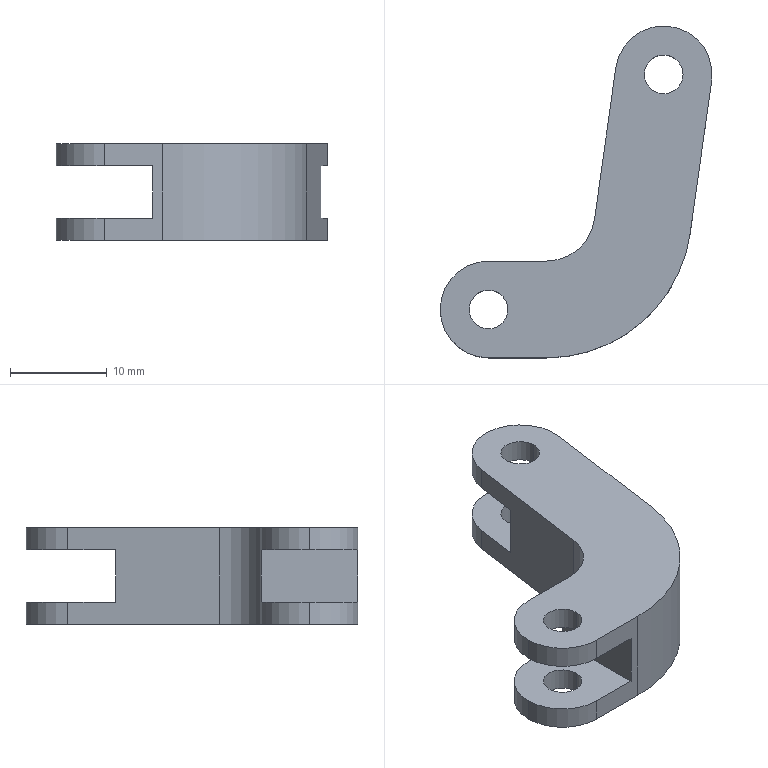Part | SolidWorks | features ICE 4, Extrusion 1 | 1 solid | 28 faces | box 28.109 x 34.304 x 10 mm | volume 3322 mm3 | cylinder 16 | plane 12 | commonest cylinder face diameters 4 x8 10 x7 30 x1
STEP:
#1=CARTESIAN_POINT('',(20.109,19.304,2.7));
#2=VERTEX_POINT('',#1);
#3=CARTESIAN_POINT('',(16.109,19.304,2.7));
#4=VERTEX_POINT('',#3);
#5=CARTESIAN_POINT('',(18.109,19.304,2.7));
#6=DIRECTION('',(0.,0.,-1.));
#7=DIRECTION('',(0.,-1.,0.));
#8=AXIS2_PLACEMENT_3D('',#5,#6,#7);
#9=CIRCLE('',#8,2.);
#10=EDGE_CURVE('',#2,#4,#9,.T.);
#11=ORIENTED_EDGE('',*,*,#10,.T.);
#12=CARTESIAN_POINT('',(16.109,19.304,5.));
#13=VERTEX_POINT('',#12);
#14=CARTESIAN_POINT('',(16.109,19.304,-26.));
#15=DIRECTION('',(0.,0.,1.));
#16=VECTOR('',#15,1000.);
#17=LINE('',#14,#16);
#18=EDGE_CURVE('',#4,#13,#17,.T.);
#19=ORIENTED_EDGE('',*,*,#18,.T.);
#20=CARTESIAN_POINT('',(20.109,19.304,5.));
#21=VERTEX_POINT('',#20);
#22=CARTESIAN_POINT('',(18.109,19.304,5.));
#23=DIRECTION('',(0.,0.,1.));
#24=DIRECTION('',(1.,0.,0.));
#25=AXIS2_PLACEMENT_3D('',#22,#23,#24);
#26=CIRCLE('',#25,2.);
#27=EDGE_CURVE('',#13,#21,#26,.T.);
#28=ORIENTED_EDGE('',*,*,#27,.T.);
#29=CARTESIAN_POINT('',(20.109,19.304,-26.));
#30=DIRECTION('',(0.,0.,1.));
#31=VECTOR('',#30,1000.);
#32=LINE('',#29,#31);
#33=EDGE_CURVE('',#2,#21,#32,.T.);
#34=ORIENTED_EDGE('',*,*,#33,.F.);
#35=EDGE_LOOP('',(#11,#19,#28,#34));
#36=FACE_OUTER_BOUND('',#35,.T.);
#37=CARTESIAN_POINT('',(18.109,19.304,-26.));
#38=DIRECTION('',(0.,0.,1.));
#39=DIRECTION('',(1.,0.,0.));
#40=AXIS2_PLACEMENT_3D('',#37,#38,#39);
#41=CYLINDRICAL_SURFACE('',#40,2.);
#42=ADVANCED_FACE('',(#36),#41,.F.);
#43=CARTESIAN_POINT('',(-2.,-5.,2.7));
#44=VERTEX_POINT('',#43);
#45=CARTESIAN_POINT('',(2.,-5.,2.7));
#46=VERTEX_POINT('',#45);
#47=CARTESIAN_POINT('',(0.,-5.,2.7));
#48=DIRECTION('',(0.,0.,1.));
#49=DIRECTION('',(0.,1.,0.));
#50=AXIS2_PLACEMENT_3D('',#47,#48,#49);
#51=CIRCLE('',#50,2.);
#52=EDGE_CURVE('',#44,#46,#51,.T.);
#53=ORIENTED_EDGE('',*,*,#52,.F.);
#54=CARTESIAN_POINT('',(-2.,-5.,5.));
#55=VERTEX_POINT('',#54);
#56=CARTESIAN_POINT('',(-2.,-5.,-5.));
#57=DIRECTION('',(0.,0.,1.));
#58=VECTOR('',#57,1000.);
#59=LINE('',#56,#58);
#60=EDGE_CURVE('',#44,#55,#59,.T.);
#61=ORIENTED_EDGE('',*,*,#60,.T.);
#62=CARTESIAN_POINT('',(2.,-5.,5.));
#63=VERTEX_POINT('',#62);
#64=CARTESIAN_POINT('',(0.,-5.,5.));
#65=DIRECTION('',(0.,0.,1.));
#66=DIRECTION('',(1.,0.,0.));
#67=AXIS2_PLACEMENT_3D('',#64,#65,#66);
#68=CIRCLE('',#67,2.);
#69=EDGE_CURVE('',#55,#63,#68,.T.);
#70=ORIENTED_EDGE('',*,*,#69,.T.);
#71=CARTESIAN_POINT('',(2.,-5.,-5.));
#72=DIRECTION('',(0.,0.,1.));
#73=VECTOR('',#72,1000.);
#74=LINE('',#71,#73);
#75=EDGE_CURVE('',#46,#63,#74,.T.);
#76=ORIENTED_EDGE('',*,*,#75,.F.);
#77=EDGE_LOOP('',(#53,#61,#70,#76));
#78=FACE_OUTER_BOUND('',#77,.T.);
#79=CARTESIAN_POINT('',(0.,-5.,-5.));
#80=DIRECTION('',(0.,0.,1.));
#81=DIRECTION('',(1.,0.,0.));
#82=AXIS2_PLACEMENT_3D('',#79,#80,#81);
#83=CYLINDRICAL_SURFACE('',#82,2.);
#84=ADVANCED_FACE('',(#78),#83,.F.);
#85=CARTESIAN_POINT('',(-2.,-5.,-5.));
#86=VERTEX_POINT('',#85);
#87=CARTESIAN_POINT('',(2.,-5.,-5.));
#88=VERTEX_POINT('',#87);
#89=CARTESIAN_POINT('',(0.,-5.,-5.));
#90=DIRECTION('',(0.,0.,1.));
#91=DIRECTION('',(1.,0.,0.));
#92=AXIS2_PLACEMENT_3D('',#89,#90,#91);
#93=CIRCLE('',#92,2.);
#94=EDGE_CURVE('',#86,#88,#93,.T.);
#95=ORIENTED_EDGE('',*,*,#94,.F.);
#96=CARTESIAN_POINT('',(-2.,-5.,-2.7));
#97=VERTEX_POINT('',#96);
#98=CARTESIAN_POINT('',(-2.,-5.,-5.));
#99=DIRECTION('',(0.,0.,1.));
#100=VECTOR('',#99,1000.);
#101=LINE('',#98,#100);
#102=EDGE_CURVE('',#86,#97,#101,.T.);
#103=ORIENTED_EDGE('',*,*,#102,.T.);
#104=CARTESIAN_POINT('',(2.,-5.,-2.7));
#105=VERTEX_POINT('',#104);
#106=CARTESIAN_POINT('',(0.,-5.,-2.7));
#107=DIRECTION('',(0.,0.,-1.));
#108=DIRECTION('',(0.,-1.,0.));
#109=AXIS2_PLACEMENT_3D('',#106,#107,#108);
#110=CIRCLE('',#109,2.);
#111=EDGE_CURVE('',#105,#97,#110,.T.);
#112=ORIENTED_EDGE('',*,*,#111,.F.);
#113=CARTESIAN_POINT('',(2.,-5.,-5.));
#114=DIRECTION('',(0.,0.,1.));
#115=VECTOR('',#114,1000.);
#116=LINE('',#113,#115);
#117=EDGE_CURVE('',#88,#105,#116,.T.);
#118=ORIENTED_EDGE('',*,*,#117,.F.);
#119=EDGE_LOOP('',(#95,#103,#112,#118));
#120=FACE_OUTER_BOUND('',#119,.T.);
#121=CARTESIAN_POINT('',(0.,-5.,-5.));
#122=DIRECTION('',(0.,0.,1.));
#123=DIRECTION('',(1.,0.,0.));
#124=AXIS2_PLACEMENT_3D('',#121,#122,#123);
#125=CYLINDRICAL_SURFACE('',#124,2.);
#126=ADVANCED_FACE('',(#120),#125,.F.);
#127=CARTESIAN_POINT('',(-5.,-5.,5.));
#128=VERTEX_POINT('',#127);
#129=CARTESIAN_POINT('',(0.,-10.,5.));
#130=VERTEX_POINT('',#129);
#131=CARTESIAN_POINT('',(0.,-5.,5.));
#132=DIRECTION('',(0.,0.,1.));
#133=DIRECTION('',(1.,0.,0.));
#134=AXIS2_PLACEMENT_3D('',#131,#132,#133);
#135=CIRCLE('',#134,5.);
#136=EDGE_CURVE('',#128,#130,#135,.T.);
#137=ORIENTED_EDGE('',*,*,#136,.F.);
#138=CARTESIAN_POINT('',(-5.,-5.,2.7));
#139=VERTEX_POINT('',#138);
#140=CARTESIAN_POINT('',(-5.,-5.,5.));
#141=DIRECTION('',(0.,0.,-1.));
#142=VECTOR('',#141,1000.);
#143=LINE('',#140,#142);
#144=EDGE_CURVE('',#128,#139,#143,.T.);
#145=ORIENTED_EDGE('',*,*,#144,.T.);
#146=CARTESIAN_POINT('',(0.,-10.,2.7));
#147=VERTEX_POINT('',#146);
#148=CARTESIAN_POINT('',(0.,-5.,2.7));
#149=DIRECTION('',(0.,0.,-1.));
#150=DIRECTION('',(0.,1.,0.));
#151=AXIS2_PLACEMENT_3D('',#148,#149,#150);
#152=CIRCLE('',#151,5.);
#153=EDGE_CURVE('',#147,#139,#152,.T.);
#154=ORIENTED_EDGE('',*,*,#153,.F.);
#155=CARTESIAN_POINT('',(0.,-10.,5.));
#156=DIRECTION('',(0.,0.,-1.));
#157=VECTOR('',#156,1000.);
#158=LINE('',#155,#157);
#159=EDGE_CURVE('',#130,#147,#158,.T.);
#160=ORIENTED_EDGE('',*,*,#159,.F.);
#161=EDGE_LOOP('',(#137,#145,#154,#160));
#162=FACE_OUTER_BOUND('',#161,.T.);
#163=CARTESIAN_POINT('',(0.,-5.,5.));
#164=DIRECTION('',(0.,0.,-1.));
#165=DIRECTION('',(-1.,0.,0.));
#166=AXIS2_PLACEMENT_3D('',#163,#164,#165);
#167=CYLINDRICAL_SURFACE('',#166,5.);
#168=ADVANCED_FACE('',(#162),#167,.T.);
#169=CARTESIAN_POINT('',(-5.,-5.,-2.7));
#170=VERTEX_POINT('',#169);
#171=CARTESIAN_POINT('',(0.,-10.,-2.7));
#172=VERTEX_POINT('',#171);
#173=CARTESIAN_POINT('',(0.,-5.,-2.7));
#174=DIRECTION('',(0.,0.,1.));
#175=DIRECTION('',(0.,-1.,0.));
#176=AXIS2_PLACEMENT_3D('',#173,#174,#175);
#177=CIRCLE('',#176,5.);
#178=EDGE_CURVE('',#170,#172,#177,.T.);
#179=ORIENTED_EDGE('',*,*,#178,.F.);
#180=CARTESIAN_POINT('',(-5.,-5.,-5.));
#181=VERTEX_POINT('',#180);
#182=CARTESIAN_POINT('',(-5.,-5.,5.));
#183=DIRECTION('',(0.,0.,-1.));
#184=VECTOR('',#183,1000.);
#185=LINE('',#182,#184);
#186=EDGE_CURVE('',#170,#181,#185,.T.);
#187=ORIENTED_EDGE('',*,*,#186,.T.);
#188=CARTESIAN_POINT('',(0.,-10.,-5.));
#189=VERTEX_POINT('',#188);
#190=CARTESIAN_POINT('',(0.,-5.,-5.));
#191=DIRECTION('',(0.,0.,1.));
#192=DIRECTION('',(1.,0.,0.));
#193=AXIS2_PLACEMENT_3D('',#190,#191,#192);
#194=CIRCLE('',#193,5.);
#195=EDGE_CURVE('',#181,#189,#194,.T.);
#196=ORIENTED_EDGE('',*,*,#195,.T.);
#197=CARTESIAN_POINT('',(0.,-10.,5.));
#198=DIRECTION('',(0.,0.,-1.));
#199=VECTOR('',#198,1000.);
#200=LINE('',#197,#199);
#201=EDGE_CURVE('',#172,#189,#200,.T.);
#202=ORIENTED_EDGE('',*,*,#201,.F.);
#203=EDGE_LOOP('',(#179,#187,#196,#202));
#204=FACE_OUTER_BOUND('',#203,.T.);
#205=CARTESIAN_POINT('',(0.,-5.,5.));
#206=DIRECTION('',(0.,0.,-1.));
#207=DIRECTION('',(-1.,0.,0.));
#208=AXIS2_PLACEMENT_3D('',#205,#206,#207);
#209=CYLINDRICAL_SURFACE('',#208,5.);
#210=ADVANCED_FACE('',(#204),#209,.T.);
#211=CARTESIAN_POINT('',(16.109,19.304,-5.));
#212=VERTEX_POINT('',#211);
#213=CARTESIAN_POINT('',(20.109,19.304,-5.));
#214=VERTEX_POINT('',#213);
#215=CARTESIAN_POINT('',(18.109,19.304,-5.));
#216=DIRECTION('',(0.,0.,1.));
#217=DIRECTION('',(1.,0.,0.));
#218=AXIS2_PLACEMENT_3D('',#215,#216,#217);
#219=CIRCLE('',#218,2.);
#220=EDGE_CURVE('',#212,#214,#219,.T.);
#221=ORIENTED_EDGE('',*,*,#220,.F.);
#222=CARTESIAN_POINT('',(16.109,19.304,-2.7));
#223=VERTEX_POINT('',#222);
#224=CARTESIAN_POINT('',(16.109,19.304,-26.));
#225=DIRECTION('',(0.,0.,1.));
#226=VECTOR('',#225,1000.);
#227=LINE('',#224,#226);
#228=EDGE_CURVE('',#212,#223,#227,.T.);
#229=ORIENTED_EDGE('',*,*,#228,.T.);
#230=CARTESIAN_POINT('',(20.109,19.304,-2.7));
#231=VERTEX_POINT('',#230);
#232=CARTESIAN_POINT('',(18.109,19.304,-2.7));
#233=DIRECTION('',(0.,0.,1.));
#234=DIRECTION('',(0.,1.,0.));
#235=AXIS2_PLACEMENT_3D('',#232,#233,#234);
#236=CIRCLE('',#235,2.);
#237=EDGE_CURVE('',#223,#231,#236,.T.);
#238=ORIENTED_EDGE('',*,*,#237,.T.);
#239=CARTESIAN_POINT('',(20.109,19.304,-26.));
#240=DIRECTION('',(0.,0.,1.));
#241=VECTOR('',#240,1000.);
#242=LINE('',#239,#241);
#243=EDGE_CURVE('',#214,#231,#242,.T.);
#244=ORIENTED_EDGE('',*,*,#243,.F.);
#245=EDGE_LOOP('',(#221,#229,#238,#244));
#246=FACE_OUTER_BOUND('',#245,.T.);
#247=CARTESIAN_POINT('',(18.109,19.304,-26.));
#248=DIRECTION('',(0.,0.,1.));
#249=DIRECTION('',(1.,0.,0.));
#250=AXIS2_PLACEMENT_3D('',#247,#248,#249);
#251=CYLINDRICAL_SURFACE('',#250,2.);
#252=ADVANCED_FACE('',(#246),#251,.F.);
#253=CARTESIAN_POINT('',(13.157,20.,-2.7));
#254=VERTEX_POINT('',#253);
#255=CARTESIAN_POINT('',(23.06,18.608,-2.7));
#256=VERTEX_POINT('',#255);
#257=CARTESIAN_POINT('',(18.109,19.304,-2.7));
#258=DIRECTION('',(0.,0.,-1.));
#259=DIRECTION('',(0.,1.,0.));
#260=AXIS2_PLACEMENT_3D('',#257,#258,#259);
#261=CIRCLE('',#260,5.);
#262=EDGE_CURVE('',#254,#256,#261,.T.);
#263=ORIENTED_EDGE('',*,*,#262,.T.);
#264=CARTESIAN_POINT('',(23.06,18.608,-5.));
#265=VERTEX_POINT('',#264);
#266=CARTESIAN_POINT('',(23.06,18.608,5.));
#267=DIRECTION('',(0.,0.,-1.));
#268=VECTOR('',#267,1000.);
#269=LINE('',#266,#268);
#270=EDGE_CURVE('',#256,#265,#269,.T.);
#271=ORIENTED_EDGE('',*,*,#270,.T.);
#272=CARTESIAN_POINT('',(13.157,20.,-5.));
#273=VERTEX_POINT('',#272);
#274=CARTESIAN_POINT('',(18.109,19.304,-5.));
#275=DIRECTION('',(0.,0.,1.));
#276=DIRECTION('',(-1.,0.,0.));
#277=AXIS2_PLACEMENT_3D('',#274,#275,#276);
#278=CIRCLE('',#277,5.);
#279=EDGE_CURVE('',#265,#273,#278,.T.);
#280=ORIENTED_EDGE('',*,*,#279,.T.);
#281=CARTESIAN_POINT('',(13.157,20.,5.));
#282=DIRECTION('',(0.,0.,-1.));
#283=VECTOR('',#282,1000.);
#284=LINE('',#281,#283);
#285=EDGE_CURVE('',#254,#273,#284,.T.);
#286=ORIENTED_EDGE('',*,*,#285,.F.);
#287=EDGE_LOOP('',(#263,#271,#280,#286));
#288=FACE_OUTER_BOUND('',#287,.T.);
#289=CARTESIAN_POINT('',(18.109,19.304,5.));
#290=DIRECTION('',(0.,0.,-1.));
#291=DIRECTION('',(-1.,0.,0.));
#292=AXIS2_PLACEMENT_3D('',#289,#290,#291);
#293=CYLINDRICAL_SURFACE('',#292,5.);
#294=ADVANCED_FACE('',(#288),#293,.T.);
#295=ORIENTED_EDGE('',*,*,#228,.F.);
#296=CARTESIAN_POINT('',(18.109,19.304,-5.));
#297=DIRECTION('',(0.,0.,1.));
#298=DIRECTION('',(1.,0.,0.));
#299=AXIS2_PLACEMENT_3D('',#296,#297,#298);
#300=CIRCLE('',#299,2.);
#301=EDGE_CURVE('',#214,#212,#300,.T.);
#302=ORIENTED_EDGE('',*,*,#301,.F.);
#303=ORIENTED_EDGE('',*,*,#243,.T.);
#304=CARTESIAN_POINT('',(18.109,19.304,-2.7));
#305=DIRECTION('',(0.,0.,1.));
#306=DIRECTION('',(0.,1.,0.));
#307=AXIS2_PLACEMENT_3D('',#304,#305,#306);
#308=CIRCLE('',#307,2.);
#309=EDGE_CURVE('',#231,#223,#308,.T.);
#310=ORIENTED_EDGE('',*,*,#309,.T.);
#311=EDGE_LOOP('',(#295,#302,#303,#310));
#312=FACE_OUTER_BOUND('',#311,.T.);
#313=CARTESIAN_POINT('',(18.109,19.304,-26.));
#314=DIRECTION('',(0.,0.,1.));
#315=DIRECTION('',(1.,0.,0.));
#316=AXIS2_PLACEMENT_3D('',#313,#314,#315);
#317=CYLINDRICAL_SURFACE('',#316,2.);
#318=ADVANCED_FACE('',(#312),#317,.F.);
#319=CARTESIAN_POINT('',(5.,0.,-2.7));
#320=VERTEX_POINT('',#319);
#321=CARTESIAN_POINT('',(0.,0.,-2.7));
#322=VERTEX_POINT('',#321);
#323=CARTESIAN_POINT('',(5.,0.,-2.7));
#324=DIRECTION('',(-1.,0.,0.));
#325=VECTOR('',#324,1000.);
#326=LINE('',#323,#325);
#327=EDGE_CURVE('',#320,#322,#326,.T.);
#328=ORIENTED_EDGE('',*,*,#327,.F.);
#329=CARTESIAN_POINT('',(5.,0.,2.7));
#330=VERTEX_POINT('',#329);
#331=CARTESIAN_POINT('',(5.,0.,-2.7));
#332=DIRECTION('',(0.,0.,1.));
#333=VECTOR('',#332,1000.);
#334=LINE('',#331,#333);
#335=EDGE_CURVE('',#320,#330,#334,.T.);
#336=ORIENTED_EDGE('',*,*,#335,.T.);
#337=CARTESIAN_POINT('',(0.,0.,2.7));
#338=VERTEX_POINT('',#337);
#339=CARTESIAN_POINT('',(5.,0.,2.7));
#340=DIRECTION('',(-1.,0.,0.));
#341=VECTOR('',#340,1000.);
#342=LINE('',#339,#341);
#343=EDGE_CURVE('',#330,#338,#342,.T.);
#344=ORIENTED_EDGE('',*,*,#343,.T.);
#345=CARTESIAN_POINT('',(0.,0.,5.));
#346=VERTEX_POINT('',#345);
#347=CARTESIAN_POINT('',(0.,0.,5.));
#348=DIRECTION('',(0.,0.,-1.));
#349=VECTOR('',#348,1000.);
#350=LINE('',#347,#349);
#351=EDGE_CURVE('',#346,#338,#350,.T.);
#352=ORIENTED_EDGE('',*,*,#351,.F.);
#353=CARTESIAN_POINT('',(6.,0.,5.));
#354=VERTEX_POINT('',#353);
#355=CARTESIAN_POINT('',(0.,0.,5.));
#356=DIRECTION('',(-1.,0.,0.));
#357=VECTOR('',#356,1000.);
#358=LINE('',#355,#357);
#359=EDGE_CURVE('',#354,#346,#358,.T.);
#360=ORIENTED_EDGE('',*,*,#359,.F.);
#361=CARTESIAN_POINT('',(6.,0.,-5.));
#362=VERTEX_POINT('',#361);
#363=CARTESIAN_POINT('',(6.,0.,5.));
#364=DIRECTION('',(0.,0.,-1.));
#365=VECTOR('',#364,1000.);
#366=LINE('',#363,#365);
#367=EDGE_CURVE('',#354,#362,#366,.T.);
#368=ORIENTED_EDGE('',*,*,#367,.T.);
#369=CARTESIAN_POINT('',(0.,0.,-5.));
#370=VERTEX_POINT('',#369);
#371=CARTESIAN_POINT('',(0.,0.,-5.));
#372=DIRECTION('',(-1.,0.,0.));
#373=VECTOR('',#372,1000.);
#374=LINE('',#371,#373);
#375=EDGE_CURVE('',#362,#370,#374,.T.);
#376=ORIENTED_EDGE('',*,*,#375,.T.);
#377=CARTESIAN_POINT('',(0.,0.,5.));
#378=DIRECTION('',(0.,0.,-1.));
#379=VECTOR('',#378,1000.);
#380=LINE('',#377,#379);
#381=EDGE_CURVE('',#322,#370,#380,.T.);
#382=ORIENTED_EDGE('',*,*,#381,.F.);
#383=EDGE_LOOP('',(#328,#336,#344,#352,#360,#368,#376,#382));
#384=FACE_OUTER_BOUND('',#383,.T.);
#385=CARTESIAN_POINT('',(0.,0.,5.));
#386=DIRECTION('',(0.,-1.,0.));
#387=DIRECTION('',(0.,0.,-1.));
#388=AXIS2_PLACEMENT_3D('',#385,#386,#387);
#389=PLANE('',#388);
#390=ADVANCED_FACE('',(#384),#389,.F.);
#391=ORIENTED_EDGE('',*,*,#186,.F.);
#392=CARTESIAN_POINT('',(0.,-5.,-2.7));
#393=DIRECTION('',(0.,0.,1.));
#394=DIRECTION('',(0.,-1.,0.));
#395=AXIS2_PLACEMENT_3D('',#392,#393,#394);
#396=CIRCLE('',#395,5.);
#397=EDGE_CURVE('',#322,#170,#396,.T.);
#398=ORIENTED_EDGE('',*,*,#397,.F.);
#399=ORIENTED_EDGE('',*,*,#381,.T.);
#400=CARTESIAN_POINT('',(0.,-5.,-5.));
#401=DIRECTION('',(0.,0.,1.));
#402=DIRECTION('',(1.,0.,0.));
#403=AXIS2_PLACEMENT_3D('',#400,#401,#402);
#404=CIRCLE('',#403,5.);
#405=EDGE_CURVE('',#370,#181,#404,.T.);
#406=ORIENTED_EDGE('',*,*,#405,.T.);
#407=EDGE_LOOP('',(#391,#398,#399,#406));
#408=FACE_OUTER_BOUND('',#407,.T.);
#409=CARTESIAN_POINT('',(0.,-5.,5.));
#410=DIRECTION('',(0.,0.,-1.));
#411=DIRECTION('',(-1.,0.,0.));
#412=AXIS2_PLACEMENT_3D('',#409,#410,#411);
#413=CYLINDRICAL_SURFACE('',#412,5.);
#414=ADVANCED_FACE('',(#408),#413,.T.);
#415=ORIENTED_EDGE('',*,*,#144,.F.);
#416=CARTESIAN_POINT('',(0.,-5.,5.));
#417=DIRECTION('',(0.,0.,1.));
#418=DIRECTION('',(1.,0.,0.));
#419=AXIS2_PLACEMENT_3D('',#416,#417,#418);
#420=CIRCLE('',#419,5.);
#421=EDGE_CURVE('',#346,#128,#420,.T.);
#422=ORIENTED_EDGE('',*,*,#421,.F.);
#423=ORIENTED_EDGE('',*,*,#351,.T.);
#424=CARTESIAN_POINT('',(0.,-5.,2.7));
#425=DIRECTION('',(0.,0.,-1.));
#426=DIRECTION('',(0.,1.,0.));
#427=AXIS2_PLACEMENT_3D('',#424,#425,#426);
#428=CIRCLE('',#427,5.);
#429=EDGE_CURVE('',#139,#338,#428,.T.);
#430=ORIENTED_EDGE('',*,*,#429,.F.);
#431=EDGE_LOOP('',(#415,#422,#423,#430));
#432=FACE_OUTER_BOUND('',#431,.T.);
#433=CARTESIAN_POINT('',(0.,-5.,5.));
#434=DIRECTION('',(0.,0.,-1.));
#435=DIRECTION('',(-1.,0.,0.));
#436=AXIS2_PLACEMENT_3D('',#433,#434,#435);
#437=CYLINDRICAL_SURFACE('',#436,5.);
#438=ADVANCED_FACE('',(#432),#437,.T.);
#439=CARTESIAN_POINT('',(5.,-10.,-2.7));
#440=VERTEX_POINT('',#439);
#441=CARTESIAN_POINT('',(5.,-10.,-2.7));
#442=DIRECTION('',(-1.,0.,0.));
#443=VECTOR('',#442,1000.);
#444=LINE('',#441,#443);
#445=EDGE_CURVE('',#440,#172,#444,.T.);
#446=ORIENTED_EDGE('',*,*,#445,.T.);
#447=ORIENTED_EDGE('',*,*,#201,.T.);
#448=CARTESIAN_POINT('',(6.,-10.,-5.));
#449=VERTEX_POINT('',#448);
#450=CARTESIAN_POINT('',(0.,-10.,-5.));
#451=DIRECTION('',(1.,0.,0.));
#452=VECTOR('',#451,1000.);
#453=LINE('',#450,#452);
#454=EDGE_CURVE('',#189,#449,#453,.T.);
#455=ORIENTED_EDGE('',*,*,#454,.T.);
#456=CARTESIAN_POINT('',(6.,-10.,5.));
#457=VERTEX_POINT('',#456);
#458=CARTESIAN_POINT('',(6.,-10.,5.));
#459=DIRECTION('',(0.,0.,-1.));
#460=VECTOR('',#459,1000.);
#461=LINE('',#458,#460);
#462=EDGE_CURVE('',#457,#449,#461,.T.);
#463=ORIENTED_EDGE('',*,*,#462,.F.);
#464=CARTESIAN_POINT('',(0.,-10.,5.));
#465=DIRECTION('',(1.,0.,0.));
#466=VECTOR('',#465,1000.);
#467=LINE('',#464,#466);
#468=EDGE_CURVE('',#130,#457,#467,.T.);
#469=ORIENTED_EDGE('',*,*,#468,.F.);
#470=ORIENTED_EDGE('',*,*,#159,.T.);
#471=CARTESIAN_POINT('',(5.,-10.,2.7));
#472=VERTEX_POINT('',#471);
#473=CARTESIAN_POINT('',(5.,-10.,2.7));
#474=DIRECTION('',(-1.,0.,0.));
#475=VECTOR('',#474,1000.);
#476=LINE('',#473,#475);
#477=EDGE_CURVE('',#472,#147,#476,.T.);
#478=ORIENTED_EDGE('',*,*,#477,.F.);
#479=CARTESIAN_POINT('',(5.,-10.,-2.7));
#480=DIRECTION('',(0.,0.,-1.));
#481=VECTOR('',#480,1000.);
#482=LINE('',#479,#481);
#483=EDGE_CURVE('',#472,#440,#482,.T.);
#484=ORIENTED_EDGE('',*,*,#483,.T.);
#485=EDGE_LOOP('',(#446,#447,#455,#463,#469,#470,#478,#484));
#486=FACE_OUTER_BOUND('',#485,.T.);
#487=CARTESIAN_POINT('',(0.,-10.,5.));
#488=DIRECTION('',(0.,1.,0.));
#489=DIRECTION('',(0.,0.,1.));
#490=AXIS2_PLACEMENT_3D('',#487,#488,#489);
#491=PLANE('',#490);
#492=ADVANCED_FACE('',(#486),#491,.F.);
#493=ORIENTED_EDGE('',*,*,#102,.F.);
#494=CARTESIAN_POINT('',(0.,-5.,-5.));
#495=DIRECTION('',(0.,0.,1.));
#496=DIRECTION('',(1.,0.,0.));
#497=AXIS2_PLACEMENT_3D('',#494,#495,#496);
#498=CIRCLE('',#497,2.);
#499=EDGE_CURVE('',#88,#86,#498,.T.);
#500=ORIENTED_EDGE('',*,*,#499,.F.);
#501=ORIENTED_EDGE('',*,*,#117,.T.);
#502=CARTESIAN_POINT('',(0.,-5.,-2.7));
#503=DIRECTION('',(0.,0.,-1.));
#504=DIRECTION('',(0.,-1.,0.));
#505=AXIS2_PLACEMENT_3D('',#502,#503,#504);
#506=CIRCLE('',#505,2.);
#507=EDGE_CURVE('',#97,#105,#506,.T.);
#508=ORIENTED_EDGE('',*,*,#507,.F.);
#509=EDGE_LOOP('',(#493,#500,#501,#508));
#510=FACE_OUTER_BOUND('',#509,.T.);
#511=CARTESIAN_POINT('',(0.,-5.,-5.));
#512=DIRECTION('',(0.,0.,1.));
#513=DIRECTION('',(1.,0.,0.));
#514=AXIS2_PLACEMENT_3D('',#511,#512,#513);
#515=CYLINDRICAL_SURFACE('',#514,2.);
#516=ADVANCED_FACE('',(#510),#515,.F.);
#517=ORIENTED_EDGE('',*,*,#60,.F.);
#518=CARTESIAN_POINT('',(0.,-5.,2.7));
#519=DIRECTION('',(0.,0.,1.));
#520=DIRECTION('',(0.,1.,0.));
#521=AXIS2_PLACEMENT_3D('',#518,#519,#520);
#522=CIRCLE('',#521,2.);
#523=EDGE_CURVE('',#46,#44,#522,.T.);
#524=ORIENTED_EDGE('',*,*,#523,.F.);
#525=ORIENTED_EDGE('',*,*,#75,.T.);
#526=CARTESIAN_POINT('',(0.,-5.,5.));
#527=DIRECTION('',(0.,0.,1.));
#528=DIRECTION('',(1.,0.,0.));
#529=AXIS2_PLACEMENT_3D('',#526,#527,#528);
#530=CIRCLE('',#529,2.);
#531=EDGE_CURVE('',#63,#55,#530,.T.);
#532=ORIENTED_EDGE('',*,*,#531,.T.);
#533=EDGE_LOOP('',(#517,#524,#525,#532));
#534=FACE_OUTER_BOUND('',#533,.T.);
#535=CARTESIAN_POINT('',(0.,-5.,-5.));
#536=DIRECTION('',(0.,0.,1.));
#537=DIRECTION('',(1.,0.,0.));
#538=AXIS2_PLACEMENT_3D('',#535,#536,#537);
#539=CYLINDRICAL_SURFACE('',#538,2.);
#540=ADVANCED_FACE('',(#534),#539,.F.);
#541=CARTESIAN_POINT('',(10.951,4.304,-5.));
#542=VERTEX_POINT('',#541);
#543=CARTESIAN_POINT('',(6.,5.,-5.));
#544=DIRECTION('',(0.,0.,-1.));
#545=DIRECTION('',(1.,0.,0.));
#546=AXIS2_PLACEMENT_3D('',#543,#544,#545);
#547=CIRCLE('',#546,5.);
#548=EDGE_CURVE('',#542,#362,#547,.T.);
#549=ORIENTED_EDGE('',*,*,#548,.T.);
#550=ORIENTED_EDGE('',*,*,#367,.F.);
#551=CARTESIAN_POINT('',(10.951,4.304,5.));
#552=VERTEX_POINT('',#551);
#553=CARTESIAN_POINT('',(6.,5.,5.));
#554=DIRECTION('',(0.,0.,-1.));
#555=DIRECTION('',(1.,0.,0.));
#556=AXIS2_PLACEMENT_3D('',#553,#554,#555);
#557=CIRCLE('',#556,5.);
#558=EDGE_CURVE('',#552,#354,#557,.T.);
#559=ORIENTED_EDGE('',*,*,#558,.F.);
#560=CARTESIAN_POINT('',(10.951,4.304,5.));
#561=DIRECTION('',(0.,0.,-1.));
#562=VECTOR('',#561,1000.);
#563=LINE('',#560,#562);
#564=EDGE_CURVE('',#552,#542,#563,.T.);
#565=ORIENTED_EDGE('',*,*,#564,.T.);
#566=EDGE_LOOP('',(#549,#550,#559,#565));
#567=FACE_OUTER_BOUND('',#566,.T.);
#568=CARTESIAN_POINT('',(6.,5.,5.));
#569=DIRECTION('',(0.,0.,-1.));
#570=DIRECTION('',(-1.,0.,0.));
#571=AXIS2_PLACEMENT_3D('',#568,#569,#570);
#572=CYLINDRICAL_SURFACE('',#571,5.);
#573=ADVANCED_FACE('',(#567),#572,.F.);
#574=CARTESIAN_POINT('',(20.854,2.912,-5.));
#575=VERTEX_POINT('',#574);
#576=CARTESIAN_POINT('',(6.,5.,-5.));
#577=DIRECTION('',(0.,0.,1.));
#578=DIRECTION('',(1.,0.,0.));
#579=AXIS2_PLACEMENT_3D('',#576,#577,#578);
#580=CIRCLE('',#579,15.);
#581=EDGE_CURVE('',#449,#575,#580,.T.);
#582=ORIENTED_EDGE('',*,*,#581,.T.);
#583=CARTESIAN_POINT('',(20.854,2.912,5.));
#584=VERTEX_POINT('',#583);
#585=CARTESIAN_POINT('',(20.854,2.912,5.));
#586=DIRECTION('',(0.,0.,-1.));
#587=VECTOR('',#586,1000.);
#588=LINE('',#585,#587);
#589=EDGE_CURVE('',#584,#575,#588,.T.);
#590=ORIENTED_EDGE('',*,*,#589,.F.);
#591=CARTESIAN_POINT('',(6.,5.,5.));
#592=DIRECTION('',(0.,0.,1.));
#593=DIRECTION('',(1.,0.,0.));
#594=AXIS2_PLACEMENT_3D('',#591,#592,#593);
#595=CIRCLE('',#594,15.);
#596=EDGE_CURVE('',#457,#584,#595,.T.);
#597=ORIENTED_EDGE('',*,*,#596,.F.);
#598=ORIENTED_EDGE('',*,*,#462,.T.);
#599=EDGE_LOOP('',(#582,#590,#597,#598));
#600=FACE_OUTER_BOUND('',#599,.T.);
#601=CARTESIAN_POINT('',(6.,5.,5.));
#602=DIRECTION('',(0.,0.,-1.));
#603=DIRECTION('',(-1.,0.,0.));
#604=AXIS2_PLACEMENT_3D('',#601,#602,#603);
#605=CYLINDRICAL_SURFACE('',#604,15.);
#606=ADVANCED_FACE('',(#600),#605,.T.);
#607=ORIENTED_EDGE('',*,*,#270,.F.);
#608=CARTESIAN_POINT('',(22.364,13.657,-2.7));
#609=VERTEX_POINT('',#608);
#610=CARTESIAN_POINT('',(23.756,23.56,-2.7));
#611=DIRECTION('',(0.1392,0.9903,0.));
#612=VECTOR('',#611,1000.);
#613=LINE('',#610,#612);
#614=EDGE_CURVE('',#609,#256,#613,.T.);
#615=ORIENTED_EDGE('',*,*,#614,.F.);
#616=CARTESIAN_POINT('',(22.364,13.657,2.7));
#617=VERTEX_POINT('',#616);
#618=CARTESIAN_POINT('',(22.364,13.657,-2.7));
#619=DIRECTION('',(0.,0.,-1.));
#620=VECTOR('',#619,1000.);
#621=LINE('',#618,#620);
#622=EDGE_CURVE('',#617,#609,#621,.T.);
#623=ORIENTED_EDGE('',*,*,#622,.F.);
#624=CARTESIAN_POINT('',(23.06,18.608,2.7));
#625=VERTEX_POINT('',#624);
#626=CARTESIAN_POINT('',(23.756,23.56,2.7));
#627=DIRECTION('',(-0.1392,-0.9903,0.));
#628=VECTOR('',#627,1000.);
#629=LINE('',#626,#628);
#630=EDGE_CURVE('',#625,#617,#629,.T.);
#631=ORIENTED_EDGE('',*,*,#630,.F.);
#632=CARTESIAN_POINT('',(23.06,18.608,5.));
#633=VERTEX_POINT('',#632);
#634=CARTESIAN_POINT('',(23.06,18.608,5.));
#635=DIRECTION('',(0.,0.,-1.));
#636=VECTOR('',#635,1000.);
#637=LINE('',#634,#636);
#638=EDGE_CURVE('',#633,#625,#637,.T.);
#639=ORIENTED_EDGE('',*,*,#638,.F.);
#640=CARTESIAN_POINT('',(20.854,2.912,5.));
#641=DIRECTION('',(0.1392,0.9903,0.));
#642=VECTOR('',#641,1000.);
#643=LINE('',#640,#642);
#644=EDGE_CURVE('',#584,#633,#643,.T.);
#645=ORIENTED_EDGE('',*,*,#644,.F.);
#646=ORIENTED_EDGE('',*,*,#589,.T.);
#647=CARTESIAN_POINT('',(20.854,2.912,-5.));
#648=DIRECTION('',(0.1392,0.9903,0.));
#649=VECTOR('',#648,1000.);
#650=LINE('',#647,#649);
#651=EDGE_CURVE('',#575,#265,#650,.T.);
#652=ORIENTED_EDGE('',*,*,#651,.T.);
#653=EDGE_LOOP('',(#607,#615,#623,#631,#639,#645,#646,#652));
#654=FACE_OUTER_BOUND('',#653,.T.);
#655=CARTESIAN_POINT('',(20.854,2.912,5.));
#656=DIRECTION('',(-0.9903,0.1392,0.));
#657=DIRECTION('',(-0.1392,-0.9903,0.));
#658=AXIS2_PLACEMENT_3D('',#655,#656,#657);
#659=PLANE('',#658);
#660=ADVANCED_FACE('',(#654),#659,.F.);
#661=ORIENTED_EDGE('',*,*,#638,.T.);
#662=CARTESIAN_POINT('',(13.157,20.,2.7));
#663=VERTEX_POINT('',#662);
#664=CARTESIAN_POINT('',(18.109,19.304,2.7));
#665=DIRECTION('',(0.,0.,1.));
#666=DIRECTION('',(0.,-1.,0.));
#667=AXIS2_PLACEMENT_3D('',#664,#665,#666);
#668=CIRCLE('',#667,5.);
#669=EDGE_CURVE('',#625,#663,#668,.T.);
#670=ORIENTED_EDGE('',*,*,#669,.T.);
#671=CARTESIAN_POINT('',(13.157,20.,5.));
#672=VERTEX_POINT('',#671);
#673=CARTESIAN_POINT('',(13.157,20.,5.));
#674=DIRECTION('',(0.,0.,-1.));
#675=VECTOR('',#674,1000.);
#676=LINE('',#673,#675);
#677=EDGE_CURVE('',#672,#663,#676,.T.);
#678=ORIENTED_EDGE('',*,*,#677,.F.);
#679=CARTESIAN_POINT('',(18.109,19.304,5.));
#680=DIRECTION('',(0.,0.,1.));
#681=DIRECTION('',(-1.,0.,0.));
#682=AXIS2_PLACEMENT_3D('',#679,#680,#681);
#683=CIRCLE('',#682,5.);
#684=EDGE_CURVE('',#633,#672,#683,.T.);
#685=ORIENTED_EDGE('',*,*,#684,.F.);
#686=EDGE_LOOP('',(#661,#670,#678,#685));
#687=FACE_OUTER_BOUND('',#686,.T.);
#688=CARTESIAN_POINT('',(18.109,19.304,5.));
#689=DIRECTION('',(0.,0.,-1.));
#690=DIRECTION('',(-1.,0.,0.));
#691=AXIS2_PLACEMENT_3D('',#688,#689,#690);
#692=CYLINDRICAL_SURFACE('',#691,5.);
#693=ADVANCED_FACE('',(#687),#692,.T.);
#694=CARTESIAN_POINT('',(12.461,15.049,2.7));
#695=VERTEX_POINT('',#694);
#696=CARTESIAN_POINT('',(12.461,15.049,-2.7));
#697=VERTEX_POINT('',#696);
#698=CARTESIAN_POINT('',(12.461,15.049,5.));
#699=DIRECTION('',(0.,0.,-1.));
#700=VECTOR('',#699,1000.);
#701=LINE('',#698,#700);
#702=EDGE_CURVE('',#695,#697,#701,.T.);
#703=ORIENTED_EDGE('',*,*,#702,.T.);
#704=CARTESIAN_POINT('',(10.951,4.304,-2.7));
#705=DIRECTION('',(0.1392,0.9903,0.));
#706=VECTOR('',#705,1000.);
#707=LINE('',#704,#706);
#708=EDGE_CURVE('',#697,#254,#707,.T.);
#709=ORIENTED_EDGE('',*,*,#708,.T.);
#710=ORIENTED_EDGE('',*,*,#285,.T.);
#711=CARTESIAN_POINT('',(10.951,4.304,-5.));
#712=DIRECTION('',(-0.1392,-0.9903,0.));
#713=VECTOR('',#712,1000.);
#714=LINE('',#711,#713);
#715=EDGE_CURVE('',#273,#542,#714,.T.);
#716=ORIENTED_EDGE('',*,*,#715,.T.);
#717=ORIENTED_EDGE('',*,*,#564,.F.);
#718=CARTESIAN_POINT('',(10.951,4.304,5.));
#719=DIRECTION('',(-0.1392,-0.9903,0.));
#720=VECTOR('',#719,1000.);
#721=LINE('',#718,#720);
#722=EDGE_CURVE('',#672,#552,#721,.T.);
#723=ORIENTED_EDGE('',*,*,#722,.F.);
#724=ORIENTED_EDGE('',*,*,#677,.T.);
#725=CARTESIAN_POINT('',(10.951,4.304,2.7));
#726=DIRECTION('',(-0.1392,-0.9903,0.));
#727=VECTOR('',#726,1000.);
#728=LINE('',#725,#727);
#729=EDGE_CURVE('',#663,#695,#728,.T.);
#730=ORIENTED_EDGE('',*,*,#729,.T.);
#731=EDGE_LOOP('',(#703,#709,#710,#716,#717,#723,#724,#730));
#732=FACE_OUTER_BOUND('',#731,.T.);
#733=CARTESIAN_POINT('',(10.951,4.304,5.));
#734=DIRECTION('',(0.9903,-0.1392,0.));
#735=DIRECTION('',(0.1392,0.9903,0.));
#736=AXIS2_PLACEMENT_3D('',#733,#734,#735);
#737=PLANE('',#736);
#738=ADVANCED_FACE('',(#732),#737,.F.);
#739=CARTESIAN_POINT('',(18.109,19.304,5.));
#740=DIRECTION('',(0.,0.,1.));
#741=DIRECTION('',(1.,0.,0.));
#742=AXIS2_PLACEMENT_3D('',#739,#740,#741);
#743=CIRCLE('',#742,2.);
#744=EDGE_CURVE('',#21,#13,#743,.T.);
#745=ORIENTED_EDGE('',*,*,#744,.F.);
#746=ORIENTED_EDGE('',*,*,#27,.F.);
#747=EDGE_LOOP('',(#745,#746));
#748=FACE_BOUND('',#747,.T.);
#749=ORIENTED_EDGE('',*,*,#531,.F.);
#750=ORIENTED_EDGE('',*,*,#69,.F.);
#751=EDGE_LOOP('',(#749,#750));
#752=FACE_BOUND('',#751,.T.);
#753=ORIENTED_EDGE('',*,*,#558,.T.);
#754=ORIENTED_EDGE('',*,*,#359,.T.);
#755=ORIENTED_EDGE('',*,*,#421,.T.);
#756=ORIENTED_EDGE('',*,*,#136,.T.);
#757=ORIENTED_EDGE('',*,*,#468,.T.);
#758=ORIENTED_EDGE('',*,*,#596,.T.);
#759=ORIENTED_EDGE('',*,*,#644,.T.);
#760=ORIENTED_EDGE('',*,*,#684,.T.);
#761=ORIENTED_EDGE('',*,*,#722,.T.);
#762=EDGE_LOOP('',(#753,#754,#755,#756,#757,#758,#759,#760,#761));
#763=FACE_OUTER_BOUND('',#762,.T.);
#764=CARTESIAN_POINT('',(6.,5.,5.));
#765=DIRECTION('',(0.,0.,1.));
#766=DIRECTION('',(1.,0.,0.));
#767=AXIS2_PLACEMENT_3D('',#764,#765,#766);
#768=PLANE('',#767);
#769=ADVANCED_FACE('',(#748,#752,#763),#768,.T.);
#770=ORIENTED_EDGE('',*,*,#301,.T.);
#771=ORIENTED_EDGE('',*,*,#220,.T.);
#772=EDGE_LOOP('',(#770,#771));
#773=FACE_BOUND('',#772,.T.);
#774=ORIENTED_EDGE('',*,*,#499,.T.);
#775=ORIENTED_EDGE('',*,*,#94,.T.);
#776=EDGE_LOOP('',(#774,#775));
#777=FACE_BOUND('',#776,.T.);
#778=ORIENTED_EDGE('',*,*,#548,.F.);
#779=ORIENTED_EDGE('',*,*,#715,.F.);
#780=ORIENTED_EDGE('',*,*,#279,.F.);
#781=ORIENTED_EDGE('',*,*,#651,.F.);
#782=ORIENTED_EDGE('',*,*,#581,.F.);
#783=ORIENTED_EDGE('',*,*,#454,.F.);
#784=ORIENTED_EDGE('',*,*,#195,.F.);
#785=ORIENTED_EDGE('',*,*,#405,.F.);
#786=ORIENTED_EDGE('',*,*,#375,.F.);
#787=EDGE_LOOP('',(#778,#779,#780,#781,#782,#783,#784,#785,#786));
#788=FACE_OUTER_BOUND('',#787,.T.);
#789=CARTESIAN_POINT('',(6.,5.,-5.));
#790=DIRECTION('',(0.,0.,1.));
#791=DIRECTION('',(1.,0.,0.));
#792=AXIS2_PLACEMENT_3D('',#789,#790,#791);
#793=PLANE('',#792);
#794=ADVANCED_FACE('',(#773,#777,#788),#793,.F.);
#795=ORIENTED_EDGE('',*,*,#111,.T.);
#796=ORIENTED_EDGE('',*,*,#507,.T.);
#797=EDGE_LOOP('',(#795,#796));
#798=FACE_BOUND('',#797,.T.);
#799=ORIENTED_EDGE('',*,*,#397,.T.);
#800=ORIENTED_EDGE('',*,*,#178,.T.);
#801=ORIENTED_EDGE('',*,*,#445,.F.);
#802=CARTESIAN_POINT('',(5.,0.,-2.7));
#803=DIRECTION('',(0.,1.,0.));
#804=VECTOR('',#803,1000.);
#805=LINE('',#802,#804);
#806=EDGE_CURVE('',#440,#320,#805,.T.);
#807=ORIENTED_EDGE('',*,*,#806,.T.);
#808=ORIENTED_EDGE('',*,*,#327,.T.);
#809=EDGE_LOOP('',(#799,#800,#801,#807,#808));
#810=FACE_OUTER_BOUND('',#809,.T.);
#811=CARTESIAN_POINT('',(5.,0.,-2.7));
#812=DIRECTION('',(0.,0.,1.));
#813=DIRECTION('',(0.,-1.,0.));
#814=AXIS2_PLACEMENT_3D('',#811,#812,#813);
#815=PLANE('',#814);
#816=ADVANCED_FACE('',(#798,#810),#815,.T.);
#817=ORIENTED_EDGE('',*,*,#523,.T.);
#818=ORIENTED_EDGE('',*,*,#52,.T.);
#819=EDGE_LOOP('',(#817,#818));
#820=FACE_BOUND('',#819,.T.);
#821=ORIENTED_EDGE('',*,*,#153,.T.);
#822=ORIENTED_EDGE('',*,*,#429,.T.);
#823=ORIENTED_EDGE('',*,*,#343,.F.);
#824=CARTESIAN_POINT('',(5.,0.,2.7));
#825=DIRECTION('',(0.,-1.,0.));
#826=VECTOR('',#825,1000.);
#827=LINE('',#824,#826);
#828=EDGE_CURVE('',#330,#472,#827,.T.);
#829=ORIENTED_EDGE('',*,*,#828,.T.);
#830=ORIENTED_EDGE('',*,*,#477,.T.);
#831=EDGE_LOOP('',(#821,#822,#823,#829,#830));
#832=FACE_OUTER_BOUND('',#831,.T.);
#833=CARTESIAN_POINT('',(5.,0.,2.7));
#834=DIRECTION('',(0.,0.,-1.));
#835=DIRECTION('',(0.,1.,0.));
#836=AXIS2_PLACEMENT_3D('',#833,#834,#835);
#837=PLANE('',#836);
#838=ADVANCED_FACE('',(#820,#832),#837,.T.);
#839=ORIENTED_EDGE('',*,*,#806,.F.);
#840=ORIENTED_EDGE('',*,*,#483,.F.);
#841=ORIENTED_EDGE('',*,*,#828,.F.);
#842=ORIENTED_EDGE('',*,*,#335,.F.);
#843=EDGE_LOOP('',(#839,#840,#841,#842));
#844=FACE_OUTER_BOUND('',#843,.T.);
#845=CARTESIAN_POINT('',(5.,0.,0.));
#846=DIRECTION('',(-1.,0.,0.));
#847=DIRECTION('',(0.,0.,1.));
#848=AXIS2_PLACEMENT_3D('',#845,#846,#847);
#849=PLANE('',#848);
#850=ADVANCED_FACE('',(#844),#849,.T.);
#851=ORIENTED_EDGE('',*,*,#18,.F.);
#852=CARTESIAN_POINT('',(18.109,19.304,2.7));
#853=DIRECTION('',(0.,0.,-1.));
#854=DIRECTION('',(0.,-1.,0.));
#855=AXIS2_PLACEMENT_3D('',#852,#853,#854);
#856=CIRCLE('',#855,2.);
#857=EDGE_CURVE('',#4,#2,#856,.T.);
#858=ORIENTED_EDGE('',*,*,#857,.T.);
#859=ORIENTED_EDGE('',*,*,#33,.T.);
#860=ORIENTED_EDGE('',*,*,#744,.T.);
#861=EDGE_LOOP('',(#851,#858,#859,#860));
#862=FACE_OUTER_BOUND('',#861,.T.);
#863=CARTESIAN_POINT('',(18.109,19.304,-26.));
#864=DIRECTION('',(0.,0.,1.));
#865=DIRECTION('',(1.,0.,0.));
#866=AXIS2_PLACEMENT_3D('',#863,#864,#865);
#867=CYLINDRICAL_SURFACE('',#866,2.);
#868=ADVANCED_FACE('',(#862),#867,.F.);
#869=CARTESIAN_POINT('',(9.491,15.466,2.7));
#870=DIRECTION('',(0.9903,-0.1392,0.));
#871=VECTOR('',#870,1000.);
#872=LINE('',#869,#871);
#873=EDGE_CURVE('',#695,#617,#872,.T.);
#874=ORIENTED_EDGE('',*,*,#873,.T.);
#875=ORIENTED_EDGE('',*,*,#622,.T.);
#876=CARTESIAN_POINT('',(9.491,15.466,-2.7));
#877=DIRECTION('',(0.9903,-0.1392,0.));
#878=VECTOR('',#877,1000.);
#879=LINE('',#876,#878);
#880=EDGE_CURVE('',#697,#609,#879,.T.);
#881=ORIENTED_EDGE('',*,*,#880,.F.);
#882=ORIENTED_EDGE('',*,*,#702,.F.);
#883=EDGE_LOOP('',(#874,#875,#881,#882));
#884=FACE_OUTER_BOUND('',#883,.T.);
#885=CARTESIAN_POINT('',(9.491,15.466,-2.7));
#886=DIRECTION('',(-0.1392,-0.9903,0.));
#887=DIRECTION('',(0.9903,-0.1392,0.));
#888=AXIS2_PLACEMENT_3D('',#885,#886,#887);
#889=PLANE('',#888);
#890=ADVANCED_FACE('',(#884),#889,.F.);
#891=ORIENTED_EDGE('',*,*,#309,.F.);
#892=ORIENTED_EDGE('',*,*,#237,.F.);
#893=EDGE_LOOP('',(#891,#892));
#894=FACE_BOUND('',#893,.T.);
#895=ORIENTED_EDGE('',*,*,#262,.F.);
#896=ORIENTED_EDGE('',*,*,#708,.F.);
#897=ORIENTED_EDGE('',*,*,#880,.T.);
#898=ORIENTED_EDGE('',*,*,#614,.T.);
#899=EDGE_LOOP('',(#895,#896,#897,#898));
#900=FACE_OUTER_BOUND('',#899,.T.);
#901=CARTESIAN_POINT('',(10.882,25.369,-2.7));
#902=DIRECTION('',(0.,0.,-1.));
#903=DIRECTION('',(0.,1.,0.));
#904=AXIS2_PLACEMENT_3D('',#901,#902,#903);
#905=PLANE('',#904);
#906=ADVANCED_FACE('',(#894,#900),#905,.F.);
#907=ORIENTED_EDGE('',*,*,#10,.F.);
#908=ORIENTED_EDGE('',*,*,#857,.F.);
#909=EDGE_LOOP('',(#907,#908));
#910=FACE_BOUND('',#909,.T.);
#911=ORIENTED_EDGE('',*,*,#630,.T.);
#912=ORIENTED_EDGE('',*,*,#873,.F.);
#913=ORIENTED_EDGE('',*,*,#729,.F.);
#914=ORIENTED_EDGE('',*,*,#669,.F.);
#915=EDGE_LOOP('',(#911,#912,#913,#914));
#916=FACE_OUTER_BOUND('',#915,.T.);
#917=CARTESIAN_POINT('',(10.882,25.369,2.7));
#918=DIRECTION('',(0.,0.,1.));
#919=DIRECTION('',(0.,-1.,0.));
#920=AXIS2_PLACEMENT_3D('',#917,#918,#919);
#921=PLANE('',#920);
#922=ADVANCED_FACE('',(#910,#916),#921,.F.);
#923=CLOSED_SHELL('',(#42,#84,#126,#168,#210,#252,#294,#318,#390,#414,#438,#492,#516,#540,#573,#606,#660,#693,#738,#769,#794,#816,#838,#850,#868,#890,#906,#922));
#924=MANIFOLD_SOLID_BREP('',#923);
#925=CARTESIAN_POINT('',(0.,0.,0.));
#926=DIRECTION('',(0.,0.,1.));
#927=DIRECTION('',(1.,0.,0.));
#928=AXIS2_PLACEMENT_3D('',#925,#926,#927);
#929=(LENGTH_UNIT()NAMED_UNIT(*)SI_UNIT(.MILLI.,.METRE.));
#930=UNCERTAINTY_MEASURE_WITH_UNIT(LENGTH_MEASURE(0.00001),#929,'','');
#931=(NAMED_UNIT(*)PLANE_ANGLE_UNIT()SI_UNIT($,.RADIAN.));
#932=(NAMED_UNIT(*)SI_UNIT($,.STERADIAN.)SOLID_ANGLE_UNIT());
#933=(GEOMETRIC_REPRESENTATION_CONTEXT(3)GLOBAL_UNCERTAINTY_ASSIGNED_CONTEXT((#930))GLOBAL_UNIT_ASSIGNED_CONTEXT((#929,#931,#932))REPRESENTATION_CONTEXT('',''));
#934=ADVANCED_BREP_SHAPE_REPRESENTATION('',(#924,#928),#933);